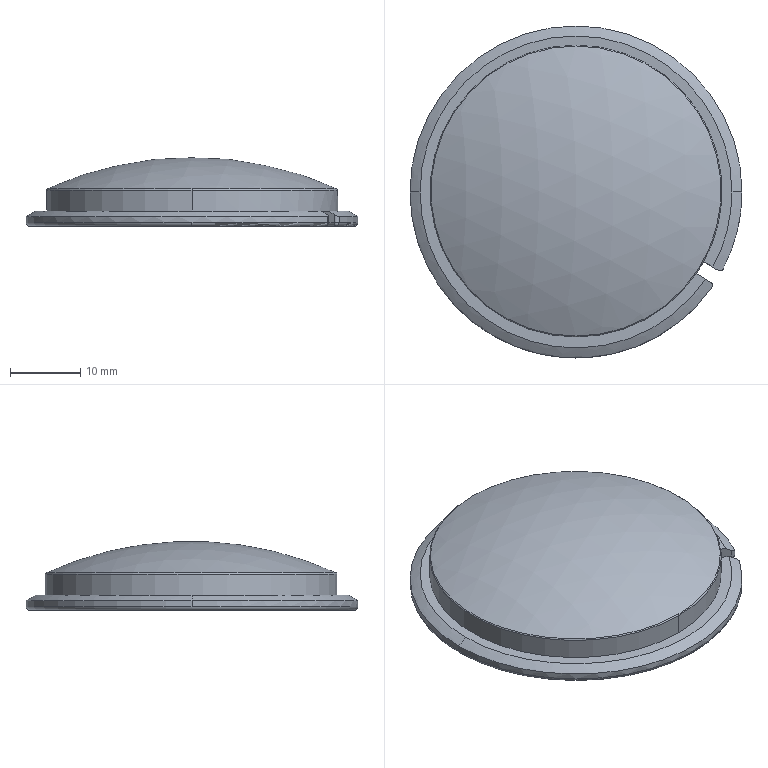Part | SolidWorks | features BaseBody 1 | 1 solid | 32 faces | box 47.34 x 47.34 x 9.8 mm | volume 4396 mm3 | torus 12 | cylinder 12 | plane 4 | sphere 4 | commonest cylinder face diameters 1 x5 47.34 x3 37.6 x2 41.6 x2
STEP:
#1=CARTESIAN_POINT('',(-125.381,-12.906,0.4856));
#2=VERTEX_POINT('',#1);
#3=CARTESIAN_POINT('',(-125.381,28.46,0.4856));
#4=VERTEX_POINT('',#3);
#5=CARTESIAN_POINT('',(-125.381,7.777,0.4856));
#6=DIRECTION('',(0.,0.,1.));
#7=DIRECTION('',(0.,1.,0.));
#8=AXIS2_PLACEMENT_3D('',#5,#6,#7);
#9=CIRCLE('',#8,20.683);
#10=EDGE_CURVE('',#2,#4,#9,.T.);
#11=ORIENTED_EDGE('',*,*,#10,.F.);
#12=CARTESIAN_POINT('',(-125.381,-13.023,0.3035));
#13=VERTEX_POINT('',#12);
#14=CARTESIAN_POINT('',(-125.381,-12.823,0.3035));
#15=DIRECTION('',(1.,0.,0.));
#16=DIRECTION('',(0.,1.,0.));
#17=AXIS2_PLACEMENT_3D('',#14,#15,#16);
#18=CIRCLE('',#17,0.2);
#19=EDGE_CURVE('',#2,#13,#18,.T.);
#20=ORIENTED_EDGE('',*,*,#19,.T.);
#21=CARTESIAN_POINT('',(-125.381,28.577,0.3035));
#22=VERTEX_POINT('',#21);
#23=CARTESIAN_POINT('',(-125.381,7.777,0.3035));
#24=DIRECTION('',(0.,0.,1.));
#25=DIRECTION('',(0.,-1.,0.));
#26=AXIS2_PLACEMENT_3D('',#23,#24,#25);
#27=CIRCLE('',#26,20.8);
#28=EDGE_CURVE('',#13,#22,#27,.T.);
#29=ORIENTED_EDGE('',*,*,#28,.T.);
#30=CARTESIAN_POINT('',(-125.381,28.377,0.3035));
#31=DIRECTION('',(-1.,0.,0.));
#32=DIRECTION('',(0.,0.,1.));
#33=AXIS2_PLACEMENT_3D('',#30,#31,#32);
#34=CIRCLE('',#33,0.2);
#35=EDGE_CURVE('',#4,#22,#34,.T.);
#36=ORIENTED_EDGE('',*,*,#35,.F.);
#37=EDGE_LOOP('',(#11,#20,#29,#36));
#38=FACE_OUTER_BOUND('',#37,.T.);
#39=CARTESIAN_POINT('',(-125.381,7.777,0.3035));
#40=DIRECTION('',(0.,0.,-1.));
#41=DIRECTION('',(0.,1.,0.));
#42=AXIS2_PLACEMENT_3D('',#39,#40,#41);
#43=TOROIDAL_SURFACE('',#42,20.6,0.2);
#44=ADVANCED_FACE('',(#38),#43,.T.);
#45=ORIENTED_EDGE('',*,*,#28,.F.);
#46=CARTESIAN_POINT('',(-125.381,-13.023,-2.679));
#47=VERTEX_POINT('',#46);
#48=CARTESIAN_POINT('',(-125.381,-13.023,4.965));
#49=DIRECTION('',(0.,0.,-1.));
#50=VECTOR('',#49,1000.);
#51=LINE('',#48,#50);
#52=EDGE_CURVE('',#13,#47,#51,.T.);
#53=ORIENTED_EDGE('',*,*,#52,.T.);
#54=CARTESIAN_POINT('',(-108.216,-3.971,-2.679));
#55=VERTEX_POINT('',#54);
#56=CARTESIAN_POINT('',(-125.381,7.777,-2.679));
#57=DIRECTION('',(0.,0.,1.));
#58=DIRECTION('',(0.,1.,0.));
#59=AXIS2_PLACEMENT_3D('',#56,#57,#58);
#60=CIRCLE('',#59,20.8);
#61=EDGE_CURVE('',#47,#55,#60,.T.);
#62=ORIENTED_EDGE('',*,*,#61,.T.);
#63=CARTESIAN_POINT('',(-108.216,-3.971,-4.336));
#64=VERTEX_POINT('',#63);
#65=CARTESIAN_POINT('',(-108.216,-3.971,-16.89));
#66=DIRECTION('',(0.,0.,-1.));
#67=VECTOR('',#66,1000.);
#68=LINE('',#65,#67);
#69=EDGE_CURVE('',#55,#64,#68,.T.);
#70=ORIENTED_EDGE('',*,*,#69,.T.);
#71=CARTESIAN_POINT('',(-108.504,-4.381,-4.836));
#72=VERTEX_POINT('',#71);
#73=CARTESIAN_POINT('',(-108.504,-4.381,-4.836));
#74=CARTESIAN_POINT('',(-108.427,-4.273,-4.836));
#75=CARTESIAN_POINT('',(-108.352,-4.168,-4.782));
#76=CARTESIAN_POINT('',(-108.247,-4.016,-4.598));
#77=CARTESIAN_POINT('',(-108.216,-3.971,-4.468));
#78=CARTESIAN_POINT('',(-108.216,-3.971,-4.336));
#79=B_SPLINE_CURVE_WITH_KNOTS('',3,(#73,#74,#75,#76,#77,#78),.UNSPECIFIED.,.F.,.F.,(4,2,4),(0.,0.0003909,0.0007818),.UNSPECIFIED.);
#80=EDGE_CURVE('',#72,#64,#79,.T.);
#81=ORIENTED_EDGE('',*,*,#80,.F.);
#82=CARTESIAN_POINT('',(-106.931,-1.826,-4.836));
#83=VERTEX_POINT('',#82);
#84=CARTESIAN_POINT('',(-125.381,7.777,-4.836));
#85=DIRECTION('',(0.,0.,1.));
#86=DIRECTION('',(0.,1.,0.));
#87=AXIS2_PLACEMENT_3D('',#84,#85,#86);
#88=CIRCLE('',#87,20.8);
#89=EDGE_CURVE('',#72,#83,#88,.T.);
#90=ORIENTED_EDGE('',*,*,#89,.T.);
#91=CARTESIAN_POINT('',(-107.167,-2.268,-4.336));
#92=VERTEX_POINT('',#91);
#93=CARTESIAN_POINT('',(-107.167,-2.268,-4.336));
#94=CARTESIAN_POINT('',(-107.167,-2.268,-4.468));
#95=CARTESIAN_POINT('',(-107.141,-2.22,-4.598));
#96=CARTESIAN_POINT('',(-107.053,-2.058,-4.782));
#97=CARTESIAN_POINT('',(-106.992,-1.944,-4.836));
#98=CARTESIAN_POINT('',(-106.931,-1.826,-4.836));
#99=B_SPLINE_CURVE_WITH_KNOTS('',3,(#93,#94,#95,#96,#97,#98),.UNSPECIFIED.,.F.,.F.,(4,2,4),(0.,0.0003909,0.0007818),.UNSPECIFIED.);
#100=EDGE_CURVE('',#92,#83,#99,.T.);
#101=ORIENTED_EDGE('',*,*,#100,.F.);
#102=CARTESIAN_POINT('',(-107.167,-2.268,-2.679));
#103=VERTEX_POINT('',#102);
#104=CARTESIAN_POINT('',(-107.167,-2.268,-16.89));
#105=DIRECTION('',(0.,0.,1.));
#106=VECTOR('',#105,1000.);
#107=LINE('',#104,#106);
#108=EDGE_CURVE('',#92,#103,#107,.T.);
#109=ORIENTED_EDGE('',*,*,#108,.T.);
#110=CARTESIAN_POINT('',(-125.381,28.577,-2.679));
#111=VERTEX_POINT('',#110);
#112=CARTESIAN_POINT('',(-125.381,7.777,-2.679));
#113=DIRECTION('',(0.,0.,1.));
#114=DIRECTION('',(0.,1.,0.));
#115=AXIS2_PLACEMENT_3D('',#112,#113,#114);
#116=CIRCLE('',#115,20.8);
#117=EDGE_CURVE('',#103,#111,#116,.T.);
#118=ORIENTED_EDGE('',*,*,#117,.T.);
#119=CARTESIAN_POINT('',(-125.381,28.577,4.965));
#120=DIRECTION('',(0.,0.,-1.));
#121=VECTOR('',#120,1000.);
#122=LINE('',#119,#121);
#123=EDGE_CURVE('',#22,#111,#122,.T.);
#124=ORIENTED_EDGE('',*,*,#123,.F.);
#125=EDGE_LOOP('',(#45,#53,#62,#70,#81,#90,#101,#109,#118,#124));
#126=FACE_OUTER_BOUND('',#125,.T.);
#127=CARTESIAN_POINT('',(-125.381,7.777,4.965));
#128=DIRECTION('',(0.,0.,-1.));
#129=DIRECTION('',(0.,1.,0.));
#130=AXIS2_PLACEMENT_3D('',#127,#128,#129);
#131=CYLINDRICAL_SURFACE('',#130,20.8);
#132=ADVANCED_FACE('',(#126),#131,.T.);
#133=CARTESIAN_POINT('',(-125.381,-11.023,-2.836));
#134=VERTEX_POINT('',#133);
#135=CARTESIAN_POINT('',(-125.381,26.577,-2.836));
#136=VERTEX_POINT('',#135);
#137=CARTESIAN_POINT('',(-125.381,7.777,-2.836));
#138=DIRECTION('',(0.,0.,1.));
#139=DIRECTION('',(0.,-1.,0.));
#140=AXIS2_PLACEMENT_3D('',#137,#138,#139);
#141=CIRCLE('',#140,18.8);
#142=EDGE_CURVE('',#134,#136,#141,.T.);
#143=ORIENTED_EDGE('',*,*,#142,.T.);
#144=CARTESIAN_POINT('',(-125.381,28.577,-4.836));
#145=VERTEX_POINT('',#144);
#146=CARTESIAN_POINT('',(-125.381,28.577,-2.836));
#147=DIRECTION('',(1.,0.,0.));
#148=DIRECTION('',(0.,1.,0.));
#149=AXIS2_PLACEMENT_3D('',#146,#147,#148);
#150=CIRCLE('',#149,2.);
#151=EDGE_CURVE('',#136,#145,#150,.T.);
#152=ORIENTED_EDGE('',*,*,#151,.T.);
#153=CARTESIAN_POINT('',(-125.381,7.777,-4.836));
#154=DIRECTION('',(0.,0.,-1.));
#155=DIRECTION('',(0.,-1.,0.));
#156=AXIS2_PLACEMENT_3D('',#153,#154,#155);
#157=CIRCLE('',#156,20.8);
#158=EDGE_CURVE('',#145,#83,#157,.T.);
#159=ORIENTED_EDGE('',*,*,#158,.T.);
#160=ORIENTED_EDGE('',*,*,#89,.F.);
#161=CARTESIAN_POINT('',(-125.381,-13.023,-4.836));
#162=VERTEX_POINT('',#161);
#163=CARTESIAN_POINT('',(-125.381,7.777,-4.836));
#164=DIRECTION('',(0.,0.,-1.));
#165=DIRECTION('',(0.,-1.,0.));
#166=AXIS2_PLACEMENT_3D('',#163,#164,#165);
#167=CIRCLE('',#166,20.8);
#168=EDGE_CURVE('',#72,#162,#167,.T.);
#169=ORIENTED_EDGE('',*,*,#168,.T.);
#170=CARTESIAN_POINT('',(-125.381,-13.023,-2.836));
#171=DIRECTION('',(-1.,0.,0.));
#172=DIRECTION('',(0.,0.,1.));
#173=AXIS2_PLACEMENT_3D('',#170,#171,#172);
#174=CIRCLE('',#173,2.);
#175=EDGE_CURVE('',#134,#162,#174,.T.);
#176=ORIENTED_EDGE('',*,*,#175,.F.);
#177=EDGE_LOOP('',(#143,#152,#159,#160,#169,#176));
#178=FACE_OUTER_BOUND('',#177,.T.);
#179=CARTESIAN_POINT('',(-125.381,7.777,-2.836));
#180=DIRECTION('',(0.,0.,1.));
#181=DIRECTION('',(0.,-1.,0.));
#182=AXIS2_PLACEMENT_3D('',#179,#180,#181);
#183=TOROIDAL_SURFACE('',#182,20.8,2.);
#184=ADVANCED_FACE('',(#178),#183,.T.);
#185=CARTESIAN_POINT('',(-101.711,7.647,-3.467));
#186=VERTEX_POINT('',#185);
#187=CARTESIAN_POINT('',(-149.051,7.647,-3.467));
#188=VERTEX_POINT('',#187);
#189=CARTESIAN_POINT('',(-125.381,7.647,-3.467));
#190=DIRECTION('',(0.,0.,1.));
#191=DIRECTION('',(0.,-1.,0.));
#192=AXIS2_PLACEMENT_3D('',#189,#190,#191);
#193=CIRCLE('',#192,23.67);
#194=EDGE_CURVE('',#186,#188,#193,.T.);
#195=ORIENTED_EDGE('',*,*,#194,.T.);
#196=CARTESIAN_POINT('',(-147.618,7.647,-2.679));
#197=VERTEX_POINT('',#196);
#198=CARTESIAN_POINT('',(-125.251,7.647,-45.036));
#199=DIRECTION('',(0.,1.,0.));
#200=DIRECTION('',(-1.,0.,0.));
#201=AXIS2_PLACEMENT_3D('',#198,#199,#200);
#202=CIRCLE('',#201,47.9);
#203=EDGE_CURVE('',#188,#197,#202,.T.);
#204=ORIENTED_EDGE('',*,*,#203,.T.);
#205=CARTESIAN_POINT('',(-103.144,7.647,-2.679));
#206=VERTEX_POINT('',#205);
#207=CARTESIAN_POINT('',(-125.381,7.647,-2.679));
#208=DIRECTION('',(0.,0.,1.));
#209=DIRECTION('',(1.,0.,0.));
#210=AXIS2_PLACEMENT_3D('',#207,#208,#209);
#211=CIRCLE('',#210,22.237);
#212=EDGE_CURVE('',#206,#197,#211,.T.);
#213=ORIENTED_EDGE('',*,*,#212,.F.);
#214=CARTESIAN_POINT('',(-125.511,7.647,-45.036));
#215=DIRECTION('',(0.,-1.,0.));
#216=DIRECTION('',(0.,0.,-1.));
#217=AXIS2_PLACEMENT_3D('',#214,#215,#216);
#218=CIRCLE('',#217,47.9);
#219=EDGE_CURVE('',#186,#206,#218,.T.);
#220=ORIENTED_EDGE('',*,*,#219,.F.);
#221=EDGE_LOOP('',(#195,#204,#213,#220));
#222=FACE_OUTER_BOUND('',#221,.T.);
#223=CARTESIAN_POINT('',(-125.381,7.647,-45.036));
#224=DIRECTION('',(0.,0.,1.));
#225=DIRECTION('',(1.,0.,0.));
#226=AXIS2_PLACEMENT_3D('',#223,#224,#225);
#227=TOROIDAL_SURFACE('',#226,-0.1299,47.9);
#228=ADVANCED_FACE('',(#222),#227,.T.);
#229=CARTESIAN_POINT('',(-104.413,-3.336,-3.467));
#230=VERTEX_POINT('',#229);
#231=CARTESIAN_POINT('',(-125.381,7.647,-3.467));
#232=DIRECTION('',(0.,0.,1.));
#233=DIRECTION('',(0.,-1.,0.));
#234=AXIS2_PLACEMENT_3D('',#231,#232,#233);
#235=CIRCLE('',#234,23.67);
#236=EDGE_CURVE('',#230,#186,#235,.T.);
#237=ORIENTED_EDGE('',*,*,#236,.T.);
#238=ORIENTED_EDGE('',*,*,#219,.T.);
#239=CARTESIAN_POINT('',(-105.889,-3.055,-2.679));
#240=VERTEX_POINT('',#239);
#241=CARTESIAN_POINT('',(-125.381,7.647,-2.679));
#242=DIRECTION('',(0.,0.,1.));
#243=DIRECTION('',(1.,0.,0.));
#244=AXIS2_PLACEMENT_3D('',#241,#242,#243);
#245=CIRCLE('',#244,22.237);
#246=EDGE_CURVE('',#240,#206,#245,.T.);
#247=ORIENTED_EDGE('',*,*,#246,.F.);
#248=CARTESIAN_POINT('',(-105.119,-3.53,-3.169));
#249=VERTEX_POINT('',#248);
#250=CARTESIAN_POINT('',(-105.889,-3.055,-2.679));
#251=CARTESIAN_POINT('',(-105.636,-3.211,-2.836));
#252=CARTESIAN_POINT('',(-105.379,-3.369,-2.999));
#253=CARTESIAN_POINT('',(-105.119,-3.53,-3.169));
#254=B_SPLINE_CURVE_WITH_KNOTS('',3,(#250,#251,#252,#253),.UNSPECIFIED.,.F.,.F.,(4,4),(0.,1.),.UNSPECIFIED.);
#255=EDGE_CURVE('',#240,#249,#254,.T.);
#256=ORIENTED_EDGE('',*,*,#255,.T.);
#257=CARTESIAN_POINT('',(-105.119,-3.53,-3.169));
#258=CARTESIAN_POINT('',(-105.063,-3.564,-3.205));
#259=CARTESIAN_POINT('',(-105.004,-3.586,-3.24));
#260=CARTESIAN_POINT('',(-104.875,-3.608,-3.309));
#261=CARTESIAN_POINT('',(-104.808,-3.606,-3.342));
#262=CARTESIAN_POINT('',(-104.676,-3.575,-3.399));
#263=CARTESIAN_POINT('',(-104.612,-3.546,-3.423));
#264=CARTESIAN_POINT('',(-104.497,-3.459,-3.458));
#265=CARTESIAN_POINT('',(-104.448,-3.402,-3.467));
#266=CARTESIAN_POINT('',(-104.413,-3.336,-3.467));
#267=B_SPLINE_CURVE_WITH_KNOTS('',3,(#257,#258,#259,#260,#261,#262,#263,#264,#265,#266),.UNSPECIFIED.,.F.,.F.,(4,2,2,2,4),(0.,0.0002187,0.0004373,0.000656,0.0008747),.UNSPECIFIED.);
#268=EDGE_CURVE('',#249,#230,#267,.T.);
#269=ORIENTED_EDGE('',*,*,#268,.T.);
#270=EDGE_LOOP('',(#237,#238,#247,#256,#269));
#271=FACE_OUTER_BOUND('',#270,.T.);
#272=CARTESIAN_POINT('',(-125.381,7.647,-45.036));
#273=DIRECTION('',(0.,0.,1.));
#274=DIRECTION('',(1.,0.,0.));
#275=AXIS2_PLACEMENT_3D('',#272,#273,#274);
#276=TOROIDAL_SURFACE('',#275,-0.1299,47.9);
#277=ADVANCED_FACE('',(#271),#276,.T.);
#278=CARTESIAN_POINT('',(-125.381,-11.023,-1.537));
#279=VERTEX_POINT('',#278);
#280=CARTESIAN_POINT('',(-125.381,26.577,-1.537));
#281=VERTEX_POINT('',#280);
#282=CARTESIAN_POINT('',(-125.381,7.777,-1.537));
#283=DIRECTION('',(0.,0.,-1.));
#284=DIRECTION('',(0.,1.,0.));
#285=AXIS2_PLACEMENT_3D('',#282,#283,#284);
#286=CIRCLE('',#285,18.8);
#287=EDGE_CURVE('',#279,#281,#286,.T.);
#288=ORIENTED_EDGE('',*,*,#287,.F.);
#289=CARTESIAN_POINT('',(-125.381,-11.023,4.965));
#290=DIRECTION('',(0.,0.,-1.));
#291=VECTOR('',#290,1000.);
#292=LINE('',#289,#291);
#293=EDGE_CURVE('',#279,#134,#292,.T.);
#294=ORIENTED_EDGE('',*,*,#293,.T.);
#295=CARTESIAN_POINT('',(-125.381,7.777,-2.836));
#296=DIRECTION('',(0.,0.,1.));
#297=DIRECTION('',(0.,-1.,0.));
#298=AXIS2_PLACEMENT_3D('',#295,#296,#297);
#299=CIRCLE('',#298,18.8);
#300=EDGE_CURVE('',#136,#134,#299,.T.);
#301=ORIENTED_EDGE('',*,*,#300,.F.);
#302=CARTESIAN_POINT('',(-125.381,26.577,4.965));
#303=DIRECTION('',(0.,0.,-1.));
#304=VECTOR('',#303,1000.);
#305=LINE('',#302,#304);
#306=EDGE_CURVE('',#281,#136,#305,.T.);
#307=ORIENTED_EDGE('',*,*,#306,.F.);
#308=EDGE_LOOP('',(#288,#294,#301,#307));
#309=FACE_OUTER_BOUND('',#308,.T.);
#310=CARTESIAN_POINT('',(-125.381,7.777,4.965));
#311=DIRECTION('',(0.,0.,-1.));
#312=DIRECTION('',(0.,1.,0.));
#313=AXIS2_PLACEMENT_3D('',#310,#311,#312);
#314=CYLINDRICAL_SURFACE('',#313,18.8);
#315=ADVANCED_FACE('',(#309),#314,.F.);
#316=CARTESIAN_POINT('',(-106.008,-5.953,-4.336));
#317=VERTEX_POINT('',#316);
#318=CARTESIAN_POINT('',(-105.918,-5.666,-4.336));
#319=VERTEX_POINT('',#318);
#320=CARTESIAN_POINT('',(-106.418,-5.666,-4.336));
#321=DIRECTION('',(0.,0.,1.));
#322=DIRECTION('',(1.,0.,0.));
#323=AXIS2_PLACEMENT_3D('',#320,#321,#322);
#324=CIRCLE('',#323,0.5);
#325=EDGE_CURVE('',#317,#319,#324,.T.);
#326=ORIENTED_EDGE('',*,*,#325,.T.);
#327=CARTESIAN_POINT('',(-105.918,-5.666,-3.416));
#328=VERTEX_POINT('',#327);
#329=CARTESIAN_POINT('',(-105.918,-5.666,4.5));
#330=DIRECTION('',(0.,0.,1.));
#331=VECTOR('',#330,1000.);
#332=LINE('',#329,#331);
#333=EDGE_CURVE('',#319,#328,#332,.T.);
#334=ORIENTED_EDGE('',*,*,#333,.T.);
#335=CARTESIAN_POINT('',(-106.008,-5.953,-3.467));
#336=VERTEX_POINT('',#335);
#337=CARTESIAN_POINT('',(-106.008,-5.953,-3.467));
#338=CARTESIAN_POINT('',(-105.948,-5.867,-3.467));
#339=CARTESIAN_POINT('',(-105.918,-5.766,-3.448));
#340=CARTESIAN_POINT('',(-105.918,-5.666,-3.416));
#341=B_SPLINE_CURVE_WITH_KNOTS('',3,(#337,#338,#339,#340),.UNSPECIFIED.,.F.,.F.,(4,4),(-0.0003094,0.),.UNSPECIFIED.);
#342=EDGE_CURVE('',#336,#328,#341,.T.);
#343=ORIENTED_EDGE('',*,*,#342,.F.);
#344=CARTESIAN_POINT('',(-106.008,-5.953,4.5));
#345=DIRECTION('',(0.,0.,-1.));
#346=VECTOR('',#345,1000.);
#347=LINE('',#344,#346);
#348=EDGE_CURVE('',#336,#317,#347,.T.);
#349=ORIENTED_EDGE('',*,*,#348,.T.);
#350=EDGE_LOOP('',(#326,#334,#343,#349));
#351=FACE_OUTER_BOUND('',#350,.T.);
#352=CARTESIAN_POINT('',(-106.418,-5.666,4.5));
#353=DIRECTION('',(0.,0.,1.));
#354=DIRECTION('',(1.,0.,0.));
#355=AXIS2_PLACEMENT_3D('',#352,#353,#354);
#356=CYLINDRICAL_SURFACE('',#355,0.5);
#357=ADVANCED_FACE('',(#351),#356,.T.);
#358=CARTESIAN_POINT('',(-125.381,31.317,-4.336));
#359=VERTEX_POINT('',#358);
#360=CARTESIAN_POINT('',(-149.051,7.647,-4.336));
#361=VERTEX_POINT('',#360);
#362=CARTESIAN_POINT('',(-125.381,7.647,-4.336));
#363=DIRECTION('',(0.,0.,1.));
#364=DIRECTION('',(1.,0.,0.));
#365=AXIS2_PLACEMENT_3D('',#362,#363,#364);
#366=CIRCLE('',#365,23.67);
#367=EDGE_CURVE('',#359,#361,#366,.T.);
#368=ORIENTED_EDGE('',*,*,#367,.T.);
#369=CARTESIAN_POINT('',(-149.051,7.647,4.5));
#370=DIRECTION('',(0.,0.,1.));
#371=VECTOR('',#370,1000.);
#372=LINE('',#369,#371);
#373=EDGE_CURVE('',#361,#188,#372,.T.);
#374=ORIENTED_EDGE('',*,*,#373,.T.);
#375=ORIENTED_EDGE('',*,*,#194,.F.);
#376=CARTESIAN_POINT('',(-101.711,7.647,-4.336));
#377=VERTEX_POINT('',#376);
#378=CARTESIAN_POINT('',(-101.711,7.647,4.5));
#379=DIRECTION('',(0.,0.,1.));
#380=VECTOR('',#379,1000.);
#381=LINE('',#378,#380);
#382=EDGE_CURVE('',#377,#186,#381,.T.);
#383=ORIENTED_EDGE('',*,*,#382,.F.);
#384=CARTESIAN_POINT('',(-125.381,7.647,-4.336));
#385=DIRECTION('',(0.,0.,1.));
#386=DIRECTION('',(1.,0.,0.));
#387=AXIS2_PLACEMENT_3D('',#384,#385,#386);
#388=CIRCLE('',#387,23.67);
#389=EDGE_CURVE('',#377,#359,#388,.T.);
#390=ORIENTED_EDGE('',*,*,#389,.T.);
#391=EDGE_LOOP('',(#368,#374,#375,#383,#390));
#392=FACE_OUTER_BOUND('',#391,.T.);
#393=CARTESIAN_POINT('',(-125.381,7.647,4.5));
#394=DIRECTION('',(0.,0.,1.));
#395=DIRECTION('',(1.,0.,0.));
#396=AXIS2_PLACEMENT_3D('',#393,#394,#395);
#397=CYLINDRICAL_SURFACE('',#396,23.67);
#398=ADVANCED_FACE('',(#392),#397,.T.);
#399=CARTESIAN_POINT('',(-104.413,-3.336,-4.336));
#400=VERTEX_POINT('',#399);
#401=CARTESIAN_POINT('',(-125.381,7.647,-4.336));
#402=DIRECTION('',(0.,0.,1.));
#403=DIRECTION('',(1.,0.,0.));
#404=AXIS2_PLACEMENT_3D('',#401,#402,#403);
#405=CIRCLE('',#404,23.67);
#406=EDGE_CURVE('',#400,#377,#405,.T.);
#407=ORIENTED_EDGE('',*,*,#406,.T.);
#408=ORIENTED_EDGE('',*,*,#382,.T.);
#409=ORIENTED_EDGE('',*,*,#236,.F.);
#410=CARTESIAN_POINT('',(-104.413,-3.336,4.5));
#411=DIRECTION('',(0.,0.,-1.));
#412=VECTOR('',#411,1000.);
#413=LINE('',#410,#412);
#414=EDGE_CURVE('',#230,#400,#413,.T.);
#415=ORIENTED_EDGE('',*,*,#414,.T.);
#416=EDGE_LOOP('',(#407,#408,#409,#415));
#417=FACE_OUTER_BOUND('',#416,.T.);
#418=CARTESIAN_POINT('',(-125.381,7.647,4.5));
#419=DIRECTION('',(0.,0.,1.));
#420=DIRECTION('',(1.,0.,0.));
#421=AXIS2_PLACEMENT_3D('',#418,#419,#420);
#422=CYLINDRICAL_SURFACE('',#421,23.67);
#423=ADVANCED_FACE('',(#417),#422,.T.);
#424=CARTESIAN_POINT('',(-104.856,-3.104,-4.836));
#425=VERTEX_POINT('',#424);
#426=CARTESIAN_POINT('',(-125.381,30.817,-4.836));
#427=VERTEX_POINT('',#426);
#428=CARTESIAN_POINT('',(-125.381,7.647,-4.836));
#429=DIRECTION('',(0.,0.,1.));
#430=DIRECTION('',(0.,-1.,0.));
#431=AXIS2_PLACEMENT_3D('',#428,#429,#430);
#432=CIRCLE('',#431,23.17);
#433=EDGE_CURVE('',#425,#427,#432,.T.);
#434=ORIENTED_EDGE('',*,*,#433,.T.);
#435=CARTESIAN_POINT('',(-125.381,30.817,-4.336));
#436=DIRECTION('',(1.,0.,0.));
#437=DIRECTION('',(0.,1.,0.));
#438=AXIS2_PLACEMENT_3D('',#435,#436,#437);
#439=CIRCLE('',#438,0.5);
#440=EDGE_CURVE('',#427,#359,#439,.T.);
#441=ORIENTED_EDGE('',*,*,#440,.T.);
#442=ORIENTED_EDGE('',*,*,#389,.F.);
#443=ORIENTED_EDGE('',*,*,#406,.F.);
#444=CARTESIAN_POINT('',(-104.856,-3.104,-4.336));
#445=DIRECTION('',(0.464,0.8858,0.));
#446=DIRECTION('',(-0.8858,0.464,0.));
#447=AXIS2_PLACEMENT_3D('',#444,#445,#446);
#448=CIRCLE('',#447,0.5);
#449=EDGE_CURVE('',#400,#425,#448,.T.);
#450=ORIENTED_EDGE('',*,*,#449,.T.);
#451=EDGE_LOOP('',(#434,#441,#442,#443,#450));
#452=FACE_OUTER_BOUND('',#451,.T.);
#453=CARTESIAN_POINT('',(-125.381,7.647,-4.336));
#454=DIRECTION('',(0.,0.,1.));
#455=DIRECTION('',(0.,-1.,0.));
#456=AXIS2_PLACEMENT_3D('',#453,#454,#455);
#457=TOROIDAL_SURFACE('',#456,23.17,0.5);
#458=ADVANCED_FACE('',(#452),#457,.T.);
#459=ORIENTED_EDGE('',*,*,#440,.F.);
#460=CARTESIAN_POINT('',(-125.381,-15.523,-4.836));
#461=VERTEX_POINT('',#460);
#462=CARTESIAN_POINT('',(-125.381,7.647,-4.836));
#463=DIRECTION('',(0.,0.,1.));
#464=DIRECTION('',(0.,-1.,0.));
#465=AXIS2_PLACEMENT_3D('',#462,#463,#464);
#466=CIRCLE('',#465,23.17);
#467=EDGE_CURVE('',#427,#461,#466,.T.);
#468=ORIENTED_EDGE('',*,*,#467,.T.);
#469=CARTESIAN_POINT('',(-125.381,-16.023,-4.336));
#470=VERTEX_POINT('',#469);
#471=CARTESIAN_POINT('',(-125.381,-15.523,-4.336));
#472=DIRECTION('',(-1.,0.,0.));
#473=DIRECTION('',(0.,0.,1.));
#474=AXIS2_PLACEMENT_3D('',#471,#472,#473);
#475=CIRCLE('',#474,0.5);
#476=EDGE_CURVE('',#461,#470,#475,.T.);
#477=ORIENTED_EDGE('',*,*,#476,.T.);
#478=CARTESIAN_POINT('',(-125.381,7.647,-4.336));
#479=DIRECTION('',(0.,0.,1.));
#480=DIRECTION('',(1.,0.,0.));
#481=AXIS2_PLACEMENT_3D('',#478,#479,#480);
#482=CIRCLE('',#481,23.67);
#483=EDGE_CURVE('',#361,#470,#482,.T.);
#484=ORIENTED_EDGE('',*,*,#483,.F.);
#485=ORIENTED_EDGE('',*,*,#367,.F.);
#486=EDGE_LOOP('',(#459,#468,#477,#484,#485));
#487=FACE_OUTER_BOUND('',#486,.T.);
#488=CARTESIAN_POINT('',(-125.381,7.647,-4.336));
#489=DIRECTION('',(0.,0.,1.));
#490=DIRECTION('',(0.,-1.,0.));
#491=AXIS2_PLACEMENT_3D('',#488,#489,#490);
#492=TOROIDAL_SURFACE('',#491,23.17,0.5);
#493=ADVANCED_FACE('',(#487),#492,.T.);
#494=CARTESIAN_POINT('',(-125.381,-10.402,-0.6116));
#495=VERTEX_POINT('',#494);
#496=CARTESIAN_POINT('',(-125.381,25.956,-0.6116));
#497=VERTEX_POINT('',#496);
#498=CARTESIAN_POINT('',(-125.381,7.777,-0.6116));
#499=DIRECTION('',(0.,0.,-1.));
#500=DIRECTION('',(0.,1.,0.));
#501=AXIS2_PLACEMENT_3D('',#498,#499,#500);
#502=CIRCLE('',#501,18.179);
#503=EDGE_CURVE('',#495,#497,#502,.T.);
#504=ORIENTED_EDGE('',*,*,#503,.F.);
#505=CARTESIAN_POINT('',(-125.381,-10.023,-1.537));
#506=DIRECTION('',(1.,0.,0.));
#507=DIRECTION('',(0.,1.,0.));
#508=AXIS2_PLACEMENT_3D('',#505,#506,#507);
#509=CIRCLE('',#508,1.);
#510=EDGE_CURVE('',#495,#279,#509,.T.);
#511=ORIENTED_EDGE('',*,*,#510,.T.);
#512=ORIENTED_EDGE('',*,*,#287,.T.);
#513=CARTESIAN_POINT('',(-125.381,25.577,-1.537));
#514=DIRECTION('',(-1.,0.,0.));
#515=DIRECTION('',(0.,0.,1.));
#516=AXIS2_PLACEMENT_3D('',#513,#514,#515);
#517=CIRCLE('',#516,1.);
#518=EDGE_CURVE('',#497,#281,#517,.T.);
#519=ORIENTED_EDGE('',*,*,#518,.F.);
#520=EDGE_LOOP('',(#504,#511,#512,#519));
#521=FACE_OUTER_BOUND('',#520,.T.);
#522=CARTESIAN_POINT('',(-125.381,7.777,-1.537));
#523=DIRECTION('',(0.,0.,-1.));
#524=DIRECTION('',(0.,1.,0.));
#525=AXIS2_PLACEMENT_3D('',#522,#523,#524);
#526=TOROIDAL_SURFACE('',#525,17.8,1.);
#527=ADVANCED_FACE('',(#521),#526,.F.);
#528=CARTESIAN_POINT('',(-125.381,7.777,0.4856));
#529=DIRECTION('',(0.,0.,1.));
#530=DIRECTION('',(0.,1.,0.));
#531=AXIS2_PLACEMENT_3D('',#528,#529,#530);
#532=CIRCLE('',#531,20.683);
#533=EDGE_CURVE('',#4,#2,#532,.T.);
#534=ORIENTED_EDGE('',*,*,#533,.T.);
#535=ORIENTED_EDGE('',*,*,#10,.T.);
#536=EDGE_LOOP('',(#534,#535));
#537=FACE_OUTER_BOUND('',#536,.T.);
#538=CARTESIAN_POINT('',(-125.381,7.777,-45.036));
#539=DIRECTION('',(-0.9094,0.,0.416));
#540=DIRECTION('',(0.416,0.,0.9094));
#541=AXIS2_PLACEMENT_3D('',#538,#539,#540);
#542=SPHERICAL_SURFACE('',#541,50.);
#543=ADVANCED_FACE('',(#537),#542,.T.);
#544=ORIENTED_EDGE('',*,*,#19,.F.);
#545=ORIENTED_EDGE('',*,*,#533,.F.);
#546=ORIENTED_EDGE('',*,*,#35,.T.);
#547=CARTESIAN_POINT('',(-125.381,7.777,0.3035));
#548=DIRECTION('',(0.,0.,1.));
#549=DIRECTION('',(0.,-1.,0.));
#550=AXIS2_PLACEMENT_3D('',#547,#548,#549);
#551=CIRCLE('',#550,20.8);
#552=EDGE_CURVE('',#22,#13,#551,.T.);
#553=ORIENTED_EDGE('',*,*,#552,.T.);
#554=EDGE_LOOP('',(#544,#545,#546,#553));
#555=FACE_OUTER_BOUND('',#554,.T.);
#556=CARTESIAN_POINT('',(-125.381,7.777,0.3035));
#557=DIRECTION('',(0.,0.,-1.));
#558=DIRECTION('',(0.,1.,0.));
#559=AXIS2_PLACEMENT_3D('',#556,#557,#558);
#560=TOROIDAL_SURFACE('',#559,20.6,0.2);
#561=ADVANCED_FACE('',(#555),#560,.T.);
#562=ORIENTED_EDGE('',*,*,#52,.F.);
#563=ORIENTED_EDGE('',*,*,#552,.F.);
#564=ORIENTED_EDGE('',*,*,#123,.T.);
#565=CARTESIAN_POINT('',(-125.381,7.777,-2.679));
#566=DIRECTION('',(0.,0.,1.));
#567=DIRECTION('',(0.,1.,0.));
#568=AXIS2_PLACEMENT_3D('',#565,#566,#567);
#569=CIRCLE('',#568,20.8);
#570=EDGE_CURVE('',#111,#47,#569,.T.);
#571=ORIENTED_EDGE('',*,*,#570,.T.);
#572=EDGE_LOOP('',(#562,#563,#564,#571));
#573=FACE_OUTER_BOUND('',#572,.T.);
#574=CARTESIAN_POINT('',(-125.381,7.777,4.965));
#575=DIRECTION('',(0.,0.,-1.));
#576=DIRECTION('',(0.,1.,0.));
#577=AXIS2_PLACEMENT_3D('',#574,#575,#576);
#578=CYLINDRICAL_SURFACE('',#577,20.8);
#579=ADVANCED_FACE('',(#573),#578,.T.);
#580=CARTESIAN_POINT('',(-106.929,-4.764,-2.679));
#581=VERTEX_POINT('',#580);
#582=CARTESIAN_POINT('',(-108.216,-3.971,-2.679));
#583=DIRECTION('',(-0.8514,0.5245,0.));
#584=VECTOR('',#583,1000.);
#585=LINE('',#582,#584);
#586=EDGE_CURVE('',#581,#55,#585,.T.);
#587=ORIENTED_EDGE('',*,*,#586,.T.);
#588=ORIENTED_EDGE('',*,*,#61,.F.);
#589=ORIENTED_EDGE('',*,*,#570,.F.);
#590=ORIENTED_EDGE('',*,*,#117,.F.);
#591=CARTESIAN_POINT('',(-107.167,-2.268,-2.679));
#592=DIRECTION('',(0.8514,-0.5245,0.));
#593=VECTOR('',#592,1000.);
#594=LINE('',#591,#593);
#595=EDGE_CURVE('',#103,#240,#594,.T.);
#596=ORIENTED_EDGE('',*,*,#595,.T.);
#597=ORIENTED_EDGE('',*,*,#246,.T.);
#598=ORIENTED_EDGE('',*,*,#212,.T.);
#599=CARTESIAN_POINT('',(-125.381,7.647,-2.679));
#600=DIRECTION('',(0.,0.,1.));
#601=DIRECTION('',(1.,0.,0.));
#602=AXIS2_PLACEMENT_3D('',#599,#600,#601);
#603=CIRCLE('',#602,22.237);
#604=EDGE_CURVE('',#197,#581,#603,.T.);
#605=ORIENTED_EDGE('',*,*,#604,.T.);
#606=EDGE_LOOP('',(#587,#588,#589,#590,#596,#597,#598,#605));
#607=FACE_OUTER_BOUND('',#606,.T.);
#608=CARTESIAN_POINT('',(-125.381,-14.59,-2.679));
#609=DIRECTION('',(0.,0.,1.));
#610=DIRECTION('',(1.,0.,0.));
#611=AXIS2_PLACEMENT_3D('',#608,#609,#610);
#612=PLANE('',#611);
#613=ADVANCED_FACE('',(#607),#612,.T.);
#614=ORIENTED_EDGE('',*,*,#151,.F.);
#615=ORIENTED_EDGE('',*,*,#300,.T.);
#616=ORIENTED_EDGE('',*,*,#175,.T.);
#617=CARTESIAN_POINT('',(-125.381,-13.023,-4.836));
#618=CARTESIAN_POINT('',(-126.484,-13.023,-4.836));
#619=CARTESIAN_POINT('',(-127.54,-12.935,-4.836));
#620=CARTESIAN_POINT('',(-129.535,-12.629,-4.836));
#621=CARTESIAN_POINT('',(-130.475,-12.41,-4.836));
#622=CARTESIAN_POINT('',(-132.229,-11.885,-4.836));
#623=CARTESIAN_POINT('',(-133.044,-11.577,-4.836));
#624=CARTESIAN_POINT('',(-134.548,-10.912,-4.836));
#625=CARTESIAN_POINT('',(-135.237,-10.554,-4.836));
#626=CARTESIAN_POINT('',(-137.125,-9.452,-4.836));
#627=CARTESIAN_POINT('',(-138.144,-8.683,-4.836));
#628=CARTESIAN_POINT('',(-139.785,-7.268,-4.836));
#629=CARTESIAN_POINT('',(-140.408,-6.622,-4.836));
#630=CARTESIAN_POINT('',(-141.354,-5.565,-4.836));
#631=CARTESIAN_POINT('',(-141.677,-5.154,-4.836));
#632=CARTESIAN_POINT('',(-141.931,-4.823,-4.836));
#633=CARTESIAN_POINT('',(-141.975,-4.765,-4.836));
#634=CARTESIAN_POINT('',(-142.02,-4.705,-4.836));
#635=CARTESIAN_POINT('',(-142.031,-4.691,-4.836));
#636=CARTESIAN_POINT('',(-142.041,-4.676,-4.836));
#637=CARTESIAN_POINT('',(-142.044,-4.673,-4.836));
#638=CARTESIAN_POINT('',(-142.045,-4.672,-4.836));
#639=CARTESIAN_POINT('',(-142.045,-4.672,-4.836));
#640=CARTESIAN_POINT('',(-142.049,-4.667,-4.836));
#641=CARTESIAN_POINT('',(-142.058,-4.655,-4.836));
#642=CARTESIAN_POINT('',(-142.096,-4.603,-4.836));
#643=CARTESIAN_POINT('',(-142.25,-4.394,-4.836));
#644=CARTESIAN_POINT('',(-142.621,-3.872,-4.836));
#645=CARTESIAN_POINT('',(-142.943,-3.376,-4.836));
#646=CARTESIAN_POINT('',(-143.251,-2.87,-4.836));
#647=CARTESIAN_POINT('',(-143.401,-2.616,-4.836));
#648=CARTESIAN_POINT('',(-143.57,-2.315,-4.836));
#649=CARTESIAN_POINT('',(-143.652,-2.163,-4.836));
#650=CARTESIAN_POINT('',(-143.687,-2.098,-4.836));
#651=CARTESIAN_POINT('',(-143.711,-2.055,-4.836));
#652=CARTESIAN_POINT('',(-143.722,-2.034,-4.836));
#653=CARTESIAN_POINT('',(-143.931,-1.642,-4.836));
#654=CARTESIAN_POINT('',(-144.117,-1.267,-4.836));
#655=CARTESIAN_POINT('',(-144.335,-0.7911,-4.836));
#656=CARTESIAN_POINT('',(-144.389,-0.6718,-4.836));
#657=CARTESIAN_POINT('',(-144.444,-0.546,-4.836));
#658=CARTESIAN_POINT('',(-144.457,-0.516,-4.836));
#659=CARTESIAN_POINT('',(-144.461,-0.507,-4.836));
#660=CARTESIAN_POINT('',(-144.462,-0.504,-4.836));
#661=CARTESIAN_POINT('',(-144.463,-0.5015,-4.836));
#662=CARTESIAN_POINT('',(-144.466,-0.4952,-4.836));
#663=CARTESIAN_POINT('',(-144.478,-0.4676,-4.836));
#664=CARTESIAN_POINT('',(-144.491,-0.4371,-4.836));
#665=CARTESIAN_POINT('',(-144.549,-0.3021,-4.836));
#666=CARTESIAN_POINT('',(-144.612,-0.1519,-4.836));
#667=CARTESIAN_POINT('',(-144.768,0.2355,-4.836));
#668=CARTESIAN_POINT('',(-144.859,0.4726,-4.836));
#669=CARTESIAN_POINT('',(-144.986,0.8253,-4.836));
#670=CARTESIAN_POINT('',(-145.018,0.917,-4.836));
#671=CARTESIAN_POINT('',(-145.053,1.018,-4.836));
#672=CARTESIAN_POINT('',(-145.061,1.042,-4.836));
#673=CARTESIAN_POINT('',(-145.064,1.052,-4.836));
#674=CARTESIAN_POINT('',(-145.065,1.055,-4.836));
#675=CARTESIAN_POINT('',(-145.068,1.064,-4.836));
#676=CARTESIAN_POINT('',(-145.078,1.093,-4.836));
#677=CARTESIAN_POINT('',(-145.12,1.217,-4.836));
#678=CARTESIAN_POINT('',(-145.159,1.336,-4.836));
#679=CARTESIAN_POINT('',(-145.313,1.817,-4.836));
#680=CARTESIAN_POINT('',(-145.429,2.216,-4.836));
#681=CARTESIAN_POINT('',(-145.639,3.04,-4.836));
#682=CARTESIAN_POINT('',(-145.734,3.465,-4.836));
#683=CARTESIAN_POINT('',(-145.838,4.013,-4.836));
#684=CARTESIAN_POINT('',(-145.858,4.123,-4.836));
#685=CARTESIAN_POINT('',(-145.887,4.29,-4.836));
#686=CARTESIAN_POINT('',(-145.897,4.346,-4.836));
#687=CARTESIAN_POINT('',(-145.914,4.452,-4.836));
#688=CARTESIAN_POINT('',(-145.957,4.718,-4.836));
#689=CARTESIAN_POINT('',(-145.995,4.985,-4.836));
#690=CARTESIAN_POINT('',(-146.128,6.053,-4.836));
#691=CARTESIAN_POINT('',(-146.182,6.914,-4.836));
#692=CARTESIAN_POINT('',(-146.181,8.209,-4.836));
#693=CARTESIAN_POINT('',(-146.167,8.64,-4.836));
#694=CARTESIAN_POINT('',(-146.134,9.178,-4.836));
#695=CARTESIAN_POINT('',(-146.125,9.313,-4.836));
#696=CARTESIAN_POINT('',(-146.114,9.454,-4.836));
#697=CARTESIAN_POINT('',(-146.111,9.488,-4.836));
#698=CARTESIAN_POINT('',(-146.11,9.498,-4.836));
#699=CARTESIAN_POINT('',(-146.11,9.501,-4.836));
#700=CARTESIAN_POINT('',(-146.11,9.504,-4.836));
#701=CARTESIAN_POINT('',(-146.109,9.511,-4.836));
#702=CARTESIAN_POINT('',(-146.107,9.54,-4.836));
#703=CARTESIAN_POINT('',(-146.104,9.572,-4.836));
#704=CARTESIAN_POINT('',(-146.091,9.718,-4.836));
#705=CARTESIAN_POINT('',(-146.076,9.883,-4.836));
#706=CARTESIAN_POINT('',(-146.028,10.311,-4.836));
#707=CARTESIAN_POINT('',(-145.995,10.573,-4.836));
#708=CARTESIAN_POINT('',(-145.937,10.96,-4.836));
#709=CARTESIAN_POINT('',(-145.921,11.06,-4.836));
#710=CARTESIAN_POINT('',(-145.903,11.171,-4.836));
#711=CARTESIAN_POINT('',(-145.898,11.197,-4.836));
#712=CARTESIAN_POINT('',(-145.897,11.208,-4.836));
#713=CARTESIAN_POINT('',(-145.896,11.211,-4.836));
#714=CARTESIAN_POINT('',(-145.895,11.221,-4.836));
#715=CARTESIAN_POINT('',(-145.889,11.252,-4.836));
#716=CARTESIAN_POINT('',(-145.867,11.385,-4.836));
#717=CARTESIAN_POINT('',(-145.771,11.917,-4.836));
#718=CARTESIAN_POINT('',(-145.659,12.43,-4.836));
#719=CARTESIAN_POINT('',(-145.452,13.254,-4.836));
#720=CARTESIAN_POINT('',(-145.334,13.669,-4.836));
#721=CARTESIAN_POINT('',(-145.169,14.189,-4.836));
#722=CARTESIAN_POINT('',(-145.135,14.293,-4.836));
#723=CARTESIAN_POINT('',(-145.082,14.449,-4.836));
#724=CARTESIAN_POINT('',(-145.065,14.502,-4.836));
#725=CARTESIAN_POINT('',(-145.031,14.6,-4.836));
#726=CARTESIAN_POINT('',(-144.945,14.847,-4.836));
#727=CARTESIAN_POINT('',(-144.709,15.484,-4.836));
#728=CARTESIAN_POINT('',(-144.465,16.062,-4.836));
#729=CARTESIAN_POINT('',(-144.204,16.632,-4.836));
#730=CARTESIAN_POINT('',(-144.069,16.915,-4.836));
#731=CARTESIAN_POINT('',(-143.904,17.241,-4.836));
#732=CARTESIAN_POINT('',(-143.82,17.404,-4.836));
#733=CARTESIAN_POINT('',(-143.783,17.473,-4.836));
#734=CARTESIAN_POINT('',(-143.759,17.519,-4.836));
#735=CARTESIAN_POINT('',(-143.746,17.543,-4.836));
#736=CARTESIAN_POINT('',(-143.548,17.913,-4.836));
#737=CARTESIAN_POINT('',(-143.352,18.257,-4.836));
#738=CARTESIAN_POINT('',(-143.096,18.678,-4.836));
#739=CARTESIAN_POINT('',(-143.031,18.783,-4.836));
#740=CARTESIAN_POINT('',(-142.962,18.893,-4.836));
#741=CARTESIAN_POINT('',(-142.946,18.919,-4.836));
#742=CARTESIAN_POINT('',(-142.941,18.927,-4.836));
#743=CARTESIAN_POINT('',(-142.939,18.929,-4.836));
#744=CARTESIAN_POINT('',(-142.938,18.931,-4.836));
#745=CARTESIAN_POINT('',(-142.935,18.936,-4.836));
#746=CARTESIAN_POINT('',(-142.921,18.957,-4.836));
#747=CARTESIAN_POINT('',(-142.906,18.981,-4.836));
#748=CARTESIAN_POINT('',(-142.837,19.089,-4.836));
#749=CARTESIAN_POINT('',(-142.756,19.215,-4.836));
#750=CARTESIAN_POINT('',(-142.536,19.542,-4.836));
#751=CARTESIAN_POINT('',(-142.398,19.743,-4.836));
#752=CARTESIAN_POINT('',(-142.184,20.037,-4.836));
#753=CARTESIAN_POINT('',(-142.128,20.114,-4.836));
#754=CARTESIAN_POINT('',(-142.066,20.197,-4.836));
#755=CARTESIAN_POINT('',(-142.051,20.217,-4.836));
#756=CARTESIAN_POINT('',(-142.047,20.223,-4.836));
#757=CARTESIAN_POINT('',(-142.045,20.225,-4.836));
#758=CARTESIAN_POINT('',(-142.045,20.226,-4.836));
#759=CARTESIAN_POINT('',(-142.044,20.226,-4.836));
#760=CARTESIAN_POINT('',(-142.042,20.23,-4.836));
#761=CARTESIAN_POINT('',(-142.033,20.242,-4.836));
#762=CARTESIAN_POINT('',(-141.992,20.296,-4.836));
#763=CARTESIAN_POINT('',(-141.943,20.362,-4.836));
#764=CARTESIAN_POINT('',(-141.705,20.672,-4.836));
#765=CARTESIAN_POINT('',(-141.394,21.07,-4.836));
#766=CARTESIAN_POINT('',(-140.469,22.112,-4.836));
#767=CARTESIAN_POINT('',(-139.854,22.755,-4.836));
#768=CARTESIAN_POINT('',(-138.225,24.174,-4.836));
#769=CARTESIAN_POINT('',(-137.209,24.949,-4.836));
#770=CARTESIAN_POINT('',(-135.318,26.065,-4.836));
#771=CARTESIAN_POINT('',(-134.626,26.428,-4.836));
#772=CARTESIAN_POINT('',(-133.115,27.103,-4.836));
#773=CARTESIAN_POINT('',(-132.295,27.416,-4.836));
#774=CARTESIAN_POINT('',(-130.527,27.952,-4.836));
#775=CARTESIAN_POINT('',(-129.579,28.175,-4.836));
#776=CARTESIAN_POINT('',(-127.564,28.487,-4.836));
#777=CARTESIAN_POINT('',(-126.497,28.577,-4.836));
#778=CARTESIAN_POINT('',(-125.381,28.577,-4.836));
#779=B_SPLINE_CURVE_WITH_KNOTS('',3,(#617,#618,#619,#620,#621,#622,#623,#624,#625,#626,#627,#628,#629,#630,#631,#632,#633,#634,#635,#636,#637,#638,#639,#640,#641,#642,#643,#644,#645,#646,#647,#648,#649,#650,#651,#652,#653,#654,#655,#656,#657,#658,#659,#660,#661,#662,#663,#664,#665,#666,#667,#668,#669,#670,#671,#672,#673,#674,#675,#676,#677,#678,#679,#680,#681,#682,#683,#684,#685,#686,#687,#688,#689,#690,#691,#692,#693,#694,#695,#696,#697,#698,#699,#700,#701,#702,#703,#704,#705,#706,#707,#708,#709,#710,#711,#712,#713,#714,#715,#716,#717,#718,#719,#720,#721,#722,#723,#724,#725,#726,#727,#728,#729,#730,#731,#732,#733,#734,#735,#736,#737,#738,#739,#740,#741,#742,#743,#744,#745,#746,#747,#748,#749,#750,#751,#752,#753,#754,#755,#756,#757,#758,#759,#760,#761,#762,#763,#764,#765,#766,#767,#768,#769,#770,#771,#772,#773,#774,#775,#776,#777,#778),.UNSPECIFIED.,.F.,.F.,(4,2,2,2,2,2,2,2,2,1,1,2,2,1,1,1,1,2,1,1,1,2,2,2,1,1,2,2,1,1,2,2,2,1,1,2,2,1,1,2,2,2,2,2,1,2,2,2,1,1,2,2,1,1,2,2,2,1,1,2,2,1,1,1,2,2,2,2,1,1,2,1,1,1,2,2,2,1,1,2,2,1,1,2,2,2,1,1,2,2,1,1,1,1,2,2,2,2,2,2,2,4),(0.,0.03125,0.0625,0.09375,0.125,0.1875,0.25,0.3125,0.3281,0.332,0.333,0.3333,0.3334,0.3335,0.334,0.3359,0.3437,0.3594,0.3672,0.3711,0.373,0.374,0.375,0.3906,0.3945,0.3955,0.3958,0.3959,0.396,0.3965,0.3984,0.4062,0.4141,0.416,0.4165,0.4166,0.4167,0.417,0.418,0.4219,0.4375,0.4531,0.457,0.459,0.4609,0.4687,0.5,0.5156,0.5195,0.5205,0.5208,0.5209,0.521,0.5215,0.5234,0.5312,0.5391,0.541,0.5415,0.5416,0.5417,0.542,0.543,0.5469,0.5625,0.5781,0.582,0.584,0.5859,0.5937,0.6094,0.6172,0.6211,0.623,0.624,0.625,0.6406,0.6445,0.6455,0.6458,0.6459,0.646,0.6465,0.6484,0.6562,0.6641,0.666,0.6665,0.6666,0.6667,0.6667,0.667,0.668,0.6719,0.6875,0.75,0.8125,0.875,0.9062,0.9375,0.9687,1.),.UNSPECIFIED.);
#780=EDGE_CURVE('',#162,#145,#779,.T.);
#781=ORIENTED_EDGE('',*,*,#780,.T.);
#782=EDGE_LOOP('',(#614,#615,#616,#781));
#783=FACE_OUTER_BOUND('',#782,.T.);
#784=CARTESIAN_POINT('',(-125.381,7.777,-2.836));
#785=DIRECTION('',(0.,0.,1.));
#786=DIRECTION('',(0.,-1.,0.));
#787=AXIS2_PLACEMENT_3D('',#784,#785,#786);
#788=TOROIDAL_SURFACE('',#787,20.8,2.);
#789=ADVANCED_FACE('',(#783),#788,.T.);
#790=ORIENTED_EDGE('',*,*,#203,.F.);
#791=CARTESIAN_POINT('',(-125.381,7.647,-3.467));
#792=DIRECTION('',(0.,0.,1.));
#793=DIRECTION('',(0.,-1.,0.));
#794=AXIS2_PLACEMENT_3D('',#791,#792,#793);
#795=CIRCLE('',#794,23.67);
#796=EDGE_CURVE('',#188,#336,#795,.T.);
#797=ORIENTED_EDGE('',*,*,#796,.T.);
#798=ORIENTED_EDGE('',*,*,#342,.T.);
#799=CARTESIAN_POINT('',(-106.155,-5.24,-3.171));
#800=VERTEX_POINT('',#799);
#801=CARTESIAN_POINT('',(-105.918,-5.666,-3.416));
#802=CARTESIAN_POINT('',(-105.918,-5.484,-3.358));
#803=CARTESIAN_POINT('',(-106.014,-5.327,-3.264));
#804=CARTESIAN_POINT('',(-106.155,-5.24,-3.171));
#805=B_SPLINE_CURVE_WITH_KNOTS('',3,(#801,#802,#803,#804),.UNSPECIFIED.,.F.,.F.,(4,4),(0.,0.000563),.UNSPECIFIED.);
#806=EDGE_CURVE('',#328,#800,#805,.T.);
#807=ORIENTED_EDGE('',*,*,#806,.T.);
#808=CARTESIAN_POINT('',(-106.155,-5.24,-3.171));
#809=CARTESIAN_POINT('',(-106.417,-5.079,-3.));
#810=CARTESIAN_POINT('',(-106.675,-4.92,-2.836));
#811=CARTESIAN_POINT('',(-106.929,-4.764,-2.679));
#812=B_SPLINE_CURVE_WITH_KNOTS('',3,(#808,#809,#810,#811),.UNSPECIFIED.,.F.,.F.,(4,4),(0.,1.),.UNSPECIFIED.);
#813=EDGE_CURVE('',#800,#581,#812,.T.);
#814=ORIENTED_EDGE('',*,*,#813,.T.);
#815=ORIENTED_EDGE('',*,*,#604,.F.);
#816=EDGE_LOOP('',(#790,#797,#798,#807,#814,#815));
#817=FACE_OUTER_BOUND('',#816,.T.);
#818=CARTESIAN_POINT('',(-125.381,7.647,-45.036));
#819=DIRECTION('',(0.,0.,1.));
#820=DIRECTION('',(1.,0.,0.));
#821=AXIS2_PLACEMENT_3D('',#818,#819,#820);
#822=TOROIDAL_SURFACE('',#821,-0.1299,47.9);
#823=ADVANCED_FACE('',(#817),#822,.T.);
#824=ORIENTED_EDGE('',*,*,#780,.F.);
#825=ORIENTED_EDGE('',*,*,#168,.F.);
#826=CARTESIAN_POINT('',(-106.418,-5.666,-4.836));
#827=VERTEX_POINT('',#826);
#828=CARTESIAN_POINT('',(-106.418,-5.666,-4.836));
#829=DIRECTION('',(-0.8514,0.5245,0.));
#830=VECTOR('',#829,1000.);
#831=LINE('',#828,#830);
#832=EDGE_CURVE('',#827,#72,#831,.T.);
#833=ORIENTED_EDGE('',*,*,#832,.F.);
#834=CARTESIAN_POINT('',(-125.381,-15.523,-4.836));
#835=CARTESIAN_POINT('',(-124.469,-15.523,-4.836));
#836=CARTESIAN_POINT('',(-123.557,-15.469,-4.836));
#837=CARTESIAN_POINT('',(-122.198,-15.309,-4.836));
#838=CARTESIAN_POINT('',(-121.747,-15.242,-4.836));
#839=CARTESIAN_POINT('',(-121.073,-15.121,-4.836));
#840=CARTESIAN_POINT('',(-120.738,-15.055,-4.836));
#841=CARTESIAN_POINT('',(-120.348,-14.971,-4.836));
#842=CARTESIAN_POINT('',(-120.153,-14.926,-4.836));
#843=CARTESIAN_POINT('',(-120.056,-14.903,-4.836));
#844=CARTESIAN_POINT('',(-120.008,-14.891,-4.836));
#845=CARTESIAN_POINT('',(-119.984,-14.886,-4.836));
#846=CARTESIAN_POINT('',(-119.971,-14.883,-4.836));
#847=CARTESIAN_POINT('',(-119.966,-14.881,-4.836));
#848=CARTESIAN_POINT('',(-119.963,-14.881,-4.836));
#849=CARTESIAN_POINT('',(-119.96,-14.88,-4.836));
#850=CARTESIAN_POINT('',(-119.93,-14.873,-4.836));
#851=CARTESIAN_POINT('',(-119.801,-14.842,-4.836));
#852=CARTESIAN_POINT('',(-119.459,-14.754,-4.836));
#853=CARTESIAN_POINT('',(-119.321,-14.717,-4.836));
#854=CARTESIAN_POINT('',(-119.077,-14.649,-4.836));
#855=CARTESIAN_POINT('',(-118.989,-14.624,-4.836));
#856=CARTESIAN_POINT('',(-118.849,-14.584,-4.836));
#857=CARTESIAN_POINT('',(-118.777,-14.562,-4.836));
#858=CARTESIAN_POINT('',(-118.689,-14.536,-4.836));
#859=CARTESIAN_POINT('',(-118.644,-14.522,-4.836));
#860=CARTESIAN_POINT('',(-118.621,-14.515,-4.836));
#861=CARTESIAN_POINT('',(-118.611,-14.512,-4.836));
#862=CARTESIAN_POINT('',(-118.605,-14.51,-4.836));
#863=CARTESIAN_POINT('',(-118.6,-14.509,-4.836));
#864=CARTESIAN_POINT('',(-118.339,-14.429,-4.836));
#865=CARTESIAN_POINT('',(-118.099,-14.351,-4.836));
#866=CARTESIAN_POINT('',(-117.767,-14.237,-4.836));
#867=CARTESIAN_POINT('',(-117.661,-14.2,-4.836));
#868=CARTESIAN_POINT('',(-117.508,-14.145,-4.836));
#869=CARTESIAN_POINT('',(-117.433,-14.118,-4.836));
#870=CARTESIAN_POINT('',(-117.349,-14.087,-4.836));
#871=CARTESIAN_POINT('',(-117.308,-14.072,-4.836));
#872=CARTESIAN_POINT('',(-117.291,-14.065,-4.836));
#873=CARTESIAN_POINT('',(-117.279,-14.061,-4.836));
#874=CARTESIAN_POINT('',(-117.274,-14.059,-4.836));
#875=CARTESIAN_POINT('',(-116.827,-13.892,-4.836));
#876=CARTESIAN_POINT('',(-116.393,-13.714,-4.836));
#877=CARTESIAN_POINT('',(-115.749,-13.428,-4.836));
#878=CARTESIAN_POINT('',(-115.429,-13.28,-4.836));
#879=CARTESIAN_POINT('',(-115.061,-13.098,-4.836));
#880=CARTESIAN_POINT('',(-114.877,-13.006,-4.836));
#881=CARTESIAN_POINT('',(-114.786,-12.959,-4.836));
#882=CARTESIAN_POINT('',(-114.74,-12.935,-4.836));
#883=CARTESIAN_POINT('',(-114.718,-12.923,-4.836));
#884=CARTESIAN_POINT('',(-114.706,-12.917,-4.836));
#885=CARTESIAN_POINT('',(-114.701,-12.915,-4.836));
#886=CARTESIAN_POINT('',(-114.698,-12.913,-4.836));
#887=CARTESIAN_POINT('',(-114.695,-12.912,-4.836));
#888=CARTESIAN_POINT('',(-114.655,-12.891,-4.836));
#889=CARTESIAN_POINT('',(-114.531,-12.827,-4.836));
#890=CARTESIAN_POINT('',(-114.221,-12.659,-4.836));
#891=CARTESIAN_POINT('',(-114.097,-12.59,-4.836));
#892=CARTESIAN_POINT('',(-113.881,-12.468,-4.836));
#893=CARTESIAN_POINT('',(-113.805,-12.424,-4.836));
#894=CARTESIAN_POINT('',(-113.682,-12.353,-4.836));
#895=CARTESIAN_POINT('',(-113.619,-12.316,-4.836));
#896=CARTESIAN_POINT('',(-113.542,-12.27,-4.836));
#897=CARTESIAN_POINT('',(-113.503,-12.247,-4.836));
#898=CARTESIAN_POINT('',(-113.483,-12.235,-4.836));
#899=CARTESIAN_POINT('',(-113.475,-12.23,-4.836));
#900=CARTESIAN_POINT('',(-113.469,-12.227,-4.836));
#901=CARTESIAN_POINT('',(-113.465,-12.225,-4.836));
#902=CARTESIAN_POINT('',(-113.231,-12.084,-4.836));
#903=CARTESIAN_POINT('',(-113.017,-11.95,-4.836));
#904=CARTESIAN_POINT('',(-112.722,-11.76,-4.836));
#905=CARTESIAN_POINT('',(-112.627,-11.698,-4.836));
#906=CARTESIAN_POINT('',(-112.492,-11.608,-4.836));
#907=CARTESIAN_POINT('',(-112.427,-11.564,-4.836));
#908=CARTESIAN_POINT('',(-112.352,-11.514,-4.836));
#909=CARTESIAN_POINT('',(-112.316,-11.489,-4.836));
#910=CARTESIAN_POINT('',(-112.301,-11.478,-4.836));
#911=CARTESIAN_POINT('',(-112.29,-11.471,-4.836));
#912=CARTESIAN_POINT('',(-112.286,-11.469,-4.836));
#913=CARTESIAN_POINT('',(-111.893,-11.199,-4.836));
#914=CARTESIAN_POINT('',(-111.514,-10.922,-4.836));
#915=CARTESIAN_POINT('',(-110.958,-10.489,-4.836));
#916=CARTESIAN_POINT('',(-110.684,-10.268,-4.836));
#917=CARTESIAN_POINT('',(-110.369,-10.003,-4.836));
#918=CARTESIAN_POINT('',(-110.214,-9.869,-4.836));
#919=CARTESIAN_POINT('',(-110.136,-9.802,-4.836));
#920=CARTESIAN_POINT('',(-110.098,-9.768,-4.836));
#921=CARTESIAN_POINT('',(-110.078,-9.751,-4.836));
#922=CARTESIAN_POINT('',(-110.069,-9.742,-4.836));
#923=CARTESIAN_POINT('',(-110.065,-9.739,-4.836));
#924=CARTESIAN_POINT('',(-110.062,-9.736,-4.836));
#925=CARTESIAN_POINT('',(-110.059,-9.734,-4.836));
#926=CARTESIAN_POINT('',(-110.028,-9.706,-4.836));
#927=CARTESIAN_POINT('',(-109.926,-9.617,-4.836));
#928=CARTESIAN_POINT('',(-109.673,-9.386,-4.836));
#929=CARTESIAN_POINT('',(-109.572,-9.293,-4.836));
#930=CARTESIAN_POINT('',(-109.397,-9.127,-4.836));
#931=CARTESIAN_POINT('',(-109.334,-9.067,-4.836));
#932=CARTESIAN_POINT('',(-109.235,-8.971,-4.836));
#933=CARTESIAN_POINT('',(-109.184,-8.922,-4.836));
#934=CARTESIAN_POINT('',(-109.122,-8.861,-4.836));
#935=CARTESIAN_POINT('',(-109.09,-8.83,-4.836));
#936=CARTESIAN_POINT('',(-109.074,-8.814,-4.836));
#937=CARTESIAN_POINT('',(-109.068,-8.807,-4.836));
#938=CARTESIAN_POINT('',(-109.063,-8.802,-4.836));
#939=CARTESIAN_POINT('',(-109.06,-8.799,-4.836));
#940=CARTESIAN_POINT('',(-108.871,-8.612,-4.836));
#941=CARTESIAN_POINT('',(-108.7,-8.436,-4.836));
#942=CARTESIAN_POINT('',(-108.465,-8.188,-4.836));
#943=CARTESIAN_POINT('',(-108.391,-8.108,-4.836));
#944=CARTESIAN_POINT('',(-108.284,-7.992,-4.836));
#945=CARTESIAN_POINT('',(-108.233,-7.935,-4.836));
#946=CARTESIAN_POINT('',(-108.174,-7.871,-4.836));
#947=CARTESIAN_POINT('',(-108.146,-7.839,-4.836));
#948=CARTESIAN_POINT('',(-108.134,-7.826,-4.836));
#949=CARTESIAN_POINT('',(-108.126,-7.817,-4.836));
#950=CARTESIAN_POINT('',(-108.123,-7.813,-4.836));
#951=CARTESIAN_POINT('',(-107.509,-7.128,-4.836));
#952=CARTESIAN_POINT('',(-106.941,-6.413,-4.836));
#953=CARTESIAN_POINT('',(-106.418,-5.666,-4.836));
#954=B_SPLINE_CURVE_WITH_KNOTS('',3,(#834,#835,#836,#837,#838,#839,#840,#841,#842,#843,#844,#845,#846,#847,#848,#849,#850,#851,#852,#853,#854,#855,#856,#857,#858,#859,#860,#861,#862,#863,#864,#865,#866,#867,#868,#869,#870,#871,#872,#873,#874,#875,#876,#877,#878,#879,#880,#881,#882,#883,#884,#885,#886,#887,#888,#889,#890,#891,#892,#893,#894,#895,#896,#897,#898,#899,#900,#901,#902,#903,#904,#905,#906,#907,#908,#909,#910,#911,#912,#913,#914,#915,#916,#917,#918,#919,#920,#921,#922,#923,#924,#925,#926,#927,#928,#929,#930,#931,#932,#933,#934,#935,#936,#937,#938,#939,#940,#941,#942,#943,#944,#945,#946,#947,#948,#949,#950,#951,#952,#953),.UNSPECIFIED.,.F.,.F.,(4,2,2,1,1,1,1,1,1,1,2,2,2,2,2,1,1,1,1,2,2,2,2,1,1,1,2,2,2,1,1,1,1,1,1,1,2,2,2,2,2,1,1,1,1,2,2,2,2,1,1,1,2,2,2,1,1,1,1,1,1,1,2,2,2,2,2,1,1,1,1,2,2,2,2,1,1,1,2,2,4),(0.,0.125,0.1875,0.2187,0.2344,0.2422,0.2461,0.248,0.249,0.2495,0.2498,0.25,0.2812,0.2969,0.3047,0.3086,0.3105,0.3115,0.312,0.3123,0.3125,0.3437,0.3594,0.3672,0.3711,0.373,0.374,0.375,0.4375,0.4687,0.4844,0.4922,0.4961,0.498,0.499,0.4995,0.4998,0.5,0.5312,0.5469,0.5547,0.5586,0.5605,0.5615,0.562,0.5623,0.5625,0.5937,0.6094,0.6172,0.6211,0.623,0.624,0.625,0.6875,0.7187,0.7344,0.7422,0.7461,0.748,0.749,0.7495,0.7498,0.75,0.7812,0.7969,0.8047,0.8086,0.8105,0.8115,0.812,0.8123,0.8125,0.8437,0.8594,0.8672,0.8711,0.873,0.874,0.875,1.),.UNSPECIFIED.);
#955=EDGE_CURVE('',#461,#827,#954,.T.);
#956=ORIENTED_EDGE('',*,*,#955,.F.);
#957=ORIENTED_EDGE('',*,*,#467,.F.);
#958=ORIENTED_EDGE('',*,*,#433,.F.);
#959=CARTESIAN_POINT('',(-106.931,-1.826,-4.836));
#960=DIRECTION('',(0.8514,-0.5245,0.));
#961=VECTOR('',#960,1000.);
#962=LINE('',#959,#961);
#963=EDGE_CURVE('',#83,#425,#962,.T.);
#964=ORIENTED_EDGE('',*,*,#963,.F.);
#965=ORIENTED_EDGE('',*,*,#158,.F.);
#966=EDGE_LOOP('',(#824,#825,#833,#956,#957,#958,#964,#965));
#967=FACE_OUTER_BOUND('',#966,.T.);
#968=CARTESIAN_POINT('',(-125.381,7.777,-4.836));
#969=DIRECTION('',(0.,0.,1.));
#970=DIRECTION('',(0.,-1.,0.));
#971=AXIS2_PLACEMENT_3D('',#968,#969,#970);
#972=PLANE('',#971);
#973=ADVANCED_FACE('',(#967),#972,.F.);
#974=ORIENTED_EDGE('',*,*,#293,.F.);
#975=CARTESIAN_POINT('',(-125.381,7.777,-1.537));
#976=DIRECTION('',(0.,0.,-1.));
#977=DIRECTION('',(0.,1.,0.));
#978=AXIS2_PLACEMENT_3D('',#975,#976,#977);
#979=CIRCLE('',#978,18.8);
#980=EDGE_CURVE('',#281,#279,#979,.T.);
#981=ORIENTED_EDGE('',*,*,#980,.F.);
#982=ORIENTED_EDGE('',*,*,#306,.T.);
#983=ORIENTED_EDGE('',*,*,#142,.F.);
#984=EDGE_LOOP('',(#974,#981,#982,#983));
#985=FACE_OUTER_BOUND('',#984,.T.);
#986=CARTESIAN_POINT('',(-125.381,7.777,4.965));
#987=DIRECTION('',(0.,0.,-1.));
#988=DIRECTION('',(0.,1.,0.));
#989=AXIS2_PLACEMENT_3D('',#986,#987,#988);
#990=CYLINDRICAL_SURFACE('',#989,18.8);
#991=ADVANCED_FACE('',(#985),#990,.F.);
#992=ORIENTED_EDGE('',*,*,#333,.F.);
#993=CARTESIAN_POINT('',(-106.155,-5.24,-4.336));
#994=VERTEX_POINT('',#993);
#995=CARTESIAN_POINT('',(-106.418,-5.666,-4.336));
#996=DIRECTION('',(0.,0.,1.));
#997=DIRECTION('',(1.,0.,0.));
#998=AXIS2_PLACEMENT_3D('',#995,#996,#997);
#999=CIRCLE('',#998,0.5);
#1000=EDGE_CURVE('',#319,#994,#999,.T.);
#1001=ORIENTED_EDGE('',*,*,#1000,.T.);
#1002=CARTESIAN_POINT('',(-106.155,-5.24,-16.89));
#1003=DIRECTION('',(0.,0.,1.));
#1004=VECTOR('',#1003,1000.);
#1005=LINE('',#1002,#1004);
#1006=EDGE_CURVE('',#994,#800,#1005,.T.);
#1007=ORIENTED_EDGE('',*,*,#1006,.T.);
#1008=ORIENTED_EDGE('',*,*,#806,.F.);
#1009=EDGE_LOOP('',(#992,#1001,#1007,#1008));
#1010=FACE_OUTER_BOUND('',#1009,.T.);
#1011=CARTESIAN_POINT('',(-106.418,-5.666,4.5));
#1012=DIRECTION('',(0.,0.,1.));
#1013=DIRECTION('',(1.,0.,0.));
#1014=AXIS2_PLACEMENT_3D('',#1011,#1012,#1013);
#1015=CYLINDRICAL_SURFACE('',#1014,0.5);
#1016=ADVANCED_FACE('',(#1010),#1015,.T.);
#1017=ORIENTED_EDGE('',*,*,#373,.F.);
#1018=ORIENTED_EDGE('',*,*,#483,.T.);
#1019=CARTESIAN_POINT('',(-125.381,7.647,-4.336));
#1020=DIRECTION('',(0.,0.,1.));
#1021=DIRECTION('',(1.,0.,0.));
#1022=AXIS2_PLACEMENT_3D('',#1019,#1020,#1021);
#1023=CIRCLE('',#1022,23.67);
#1024=EDGE_CURVE('',#470,#317,#1023,.T.);
#1025=ORIENTED_EDGE('',*,*,#1024,.T.);
#1026=ORIENTED_EDGE('',*,*,#348,.F.);
#1027=ORIENTED_EDGE('',*,*,#796,.F.);
#1028=EDGE_LOOP('',(#1017,#1018,#1025,#1026,#1027));
#1029=FACE_OUTER_BOUND('',#1028,.T.);
#1030=CARTESIAN_POINT('',(-125.381,7.647,4.5));
#1031=DIRECTION('',(0.,0.,1.));
#1032=DIRECTION('',(1.,0.,0.));
#1033=AXIS2_PLACEMENT_3D('',#1030,#1031,#1032);
#1034=CYLINDRICAL_SURFACE('',#1033,23.67);
#1035=ADVANCED_FACE('',(#1029),#1034,.T.);
#1036=CARTESIAN_POINT('',(-105.119,-3.53,-4.336));
#1037=VERTEX_POINT('',#1036);
#1038=CARTESIAN_POINT('',(-104.856,-3.104,-4.336));
#1039=DIRECTION('',(0.,0.,1.));
#1040=DIRECTION('',(1.,0.,0.));
#1041=AXIS2_PLACEMENT_3D('',#1038,#1039,#1040);
#1042=CIRCLE('',#1041,0.5);
#1043=EDGE_CURVE('',#1037,#400,#1042,.T.);
#1044=ORIENTED_EDGE('',*,*,#1043,.T.);
#1045=ORIENTED_EDGE('',*,*,#414,.F.);
#1046=ORIENTED_EDGE('',*,*,#268,.F.);
#1047=CARTESIAN_POINT('',(-105.119,-3.53,-16.89));
#1048=DIRECTION('',(0.,0.,-1.));
#1049=VECTOR('',#1048,1000.);
#1050=LINE('',#1047,#1049);
#1051=EDGE_CURVE('',#249,#1037,#1050,.T.);
#1052=ORIENTED_EDGE('',*,*,#1051,.T.);
#1053=EDGE_LOOP('',(#1044,#1045,#1046,#1052));
#1054=FACE_OUTER_BOUND('',#1053,.T.);
#1055=CARTESIAN_POINT('',(-104.856,-3.104,4.5));
#1056=DIRECTION('',(0.,0.,1.));
#1057=DIRECTION('',(1.,0.,0.));
#1058=AXIS2_PLACEMENT_3D('',#1055,#1056,#1057);
#1059=CYLINDRICAL_SURFACE('',#1058,0.5);
#1060=ADVANCED_FACE('',(#1054),#1059,.T.);
#1061=ORIENTED_EDGE('',*,*,#832,.T.);
#1062=ORIENTED_EDGE('',*,*,#80,.T.);
#1063=CARTESIAN_POINT('',(-125.906,6.926,-4.336));
#1064=DIRECTION('',(0.8514,-0.5245,0.));
#1065=VECTOR('',#1064,1000.);
#1066=LINE('',#1063,#1065);
#1067=EDGE_CURVE('',#64,#994,#1066,.T.);
#1068=ORIENTED_EDGE('',*,*,#1067,.T.);
#1069=CARTESIAN_POINT('',(-106.418,-5.666,-4.336));
#1070=DIRECTION('',(-0.8514,0.5245,0.));
#1071=DIRECTION('',(-0.5245,-0.8514,0.));
#1072=AXIS2_PLACEMENT_3D('',#1069,#1070,#1071);
#1073=CIRCLE('',#1072,0.5);
#1074=EDGE_CURVE('',#994,#827,#1073,.T.);
#1075=ORIENTED_EDGE('',*,*,#1074,.T.);
#1076=EDGE_LOOP('',(#1061,#1062,#1068,#1075));
#1077=FACE_OUTER_BOUND('',#1076,.T.);
#1078=CARTESIAN_POINT('',(-126.168,6.5,-4.336));
#1079=DIRECTION('',(-0.8514,0.5245,0.));
#1080=DIRECTION('',(-0.5245,-0.8514,0.));
#1081=AXIS2_PLACEMENT_3D('',#1078,#1079,#1080);
#1082=CYLINDRICAL_SURFACE('',#1081,0.5);
#1083=ADVANCED_FACE('',(#1077),#1082,.T.);
#1084=ORIENTED_EDGE('',*,*,#476,.F.);
#1085=ORIENTED_EDGE('',*,*,#955,.T.);
#1086=CARTESIAN_POINT('',(-106.418,-5.666,-4.336));
#1087=DIRECTION('',(-0.5746,-0.8185,0.));
#1088=DIRECTION('',(0.8185,-0.5746,0.));
#1089=AXIS2_PLACEMENT_3D('',#1086,#1087,#1088);
#1090=CIRCLE('',#1089,0.5);
#1091=EDGE_CURVE('',#827,#317,#1090,.T.);
#1092=ORIENTED_EDGE('',*,*,#1091,.T.);
#1093=ORIENTED_EDGE('',*,*,#1024,.F.);
#1094=EDGE_LOOP('',(#1084,#1085,#1092,#1093));
#1095=FACE_OUTER_BOUND('',#1094,.T.);
#1096=CARTESIAN_POINT('',(-125.381,7.647,-4.336));
#1097=DIRECTION('',(0.,0.,1.));
#1098=DIRECTION('',(0.,-1.,0.));
#1099=AXIS2_PLACEMENT_3D('',#1096,#1097,#1098);
#1100=TOROIDAL_SURFACE('',#1099,23.17,0.5);
#1101=ADVANCED_FACE('',(#1095),#1100,.T.);
#1102=CARTESIAN_POINT('',(-124.857,8.628,-4.336));
#1103=DIRECTION('',(-0.8514,0.5245,0.));
#1104=VECTOR('',#1103,1000.);
#1105=LINE('',#1102,#1104);
#1106=EDGE_CURVE('',#1037,#92,#1105,.T.);
#1107=ORIENTED_EDGE('',*,*,#1106,.T.);
#1108=ORIENTED_EDGE('',*,*,#100,.T.);
#1109=ORIENTED_EDGE('',*,*,#963,.T.);
#1110=CARTESIAN_POINT('',(-104.856,-3.104,-4.336));
#1111=DIRECTION('',(-0.8514,0.5245,0.));
#1112=DIRECTION('',(0.5245,0.8514,0.));
#1113=AXIS2_PLACEMENT_3D('',#1110,#1111,#1112);
#1114=CIRCLE('',#1113,0.5);
#1115=EDGE_CURVE('',#425,#1037,#1114,.T.);
#1116=ORIENTED_EDGE('',*,*,#1115,.T.);
#1117=EDGE_LOOP('',(#1107,#1108,#1109,#1116));
#1118=FACE_OUTER_BOUND('',#1117,.T.);
#1119=CARTESIAN_POINT('',(-124.594,9.054,-4.336));
#1120=DIRECTION('',(0.8514,-0.5245,0.));
#1121=DIRECTION('',(0.5245,0.8514,0.));
#1122=AXIS2_PLACEMENT_3D('',#1119,#1120,#1121);
#1123=CYLINDRICAL_SURFACE('',#1122,0.5);
#1124=ADVANCED_FACE('',(#1118),#1123,.T.);
#1125=ORIENTED_EDGE('',*,*,#510,.F.);
#1126=CARTESIAN_POINT('',(-125.381,7.777,-0.6116));
#1127=DIRECTION('',(0.,0.,-1.));
#1128=DIRECTION('',(0.,1.,0.));
#1129=AXIS2_PLACEMENT_3D('',#1126,#1127,#1128);
#1130=CIRCLE('',#1129,18.179);
#1131=EDGE_CURVE('',#497,#495,#1130,.T.);
#1132=ORIENTED_EDGE('',*,*,#1131,.F.);
#1133=ORIENTED_EDGE('',*,*,#518,.T.);
#1134=ORIENTED_EDGE('',*,*,#980,.T.);
#1135=EDGE_LOOP('',(#1125,#1132,#1133,#1134));
#1136=FACE_OUTER_BOUND('',#1135,.T.);
#1137=CARTESIAN_POINT('',(-125.381,7.777,-1.537));
#1138=DIRECTION('',(0.,0.,-1.));
#1139=DIRECTION('',(0.,1.,0.));
#1140=AXIS2_PLACEMENT_3D('',#1137,#1138,#1139);
#1141=TOROIDAL_SURFACE('',#1140,17.8,1.);
#1142=ADVANCED_FACE('',(#1136),#1141,.F.);
#1143=ORIENTED_EDGE('',*,*,#325,.F.);
#1144=ORIENTED_EDGE('',*,*,#1091,.F.);
#1145=ORIENTED_EDGE('',*,*,#1074,.F.);
#1146=ORIENTED_EDGE('',*,*,#1000,.F.);
#1147=EDGE_LOOP('',(#1143,#1144,#1145,#1146));
#1148=FACE_OUTER_BOUND('',#1147,.T.);
#1149=CARTESIAN_POINT('',(-106.418,-5.666,-4.336));
#1150=DIRECTION('',(0.,0.,1.));
#1151=DIRECTION('',(-0.8185,0.5746,0.));
#1152=AXIS2_PLACEMENT_3D('',#1149,#1150,#1151);
#1153=SPHERICAL_SURFACE('',#1152,0.5);
#1154=ADVANCED_FACE('',(#1148),#1153,.T.);
#1155=ORIENTED_EDGE('',*,*,#1115,.F.);
#1156=ORIENTED_EDGE('',*,*,#449,.F.);
#1157=ORIENTED_EDGE('',*,*,#1043,.F.);
#1158=EDGE_LOOP('',(#1155,#1156,#1157));
#1159=FACE_OUTER_BOUND('',#1158,.T.);
#1160=CARTESIAN_POINT('',(-104.856,-3.104,-4.336));
#1161=DIRECTION('',(0.,0.,-1.));
#1162=DIRECTION('',(0.8858,-0.464,0.));
#1163=AXIS2_PLACEMENT_3D('',#1160,#1161,#1162);
#1164=SPHERICAL_SURFACE('',#1163,0.5);
#1165=ADVANCED_FACE('',(#1159),#1164,.T.);
#1166=ORIENTED_EDGE('',*,*,#586,.F.);
#1167=ORIENTED_EDGE('',*,*,#813,.F.);
#1168=ORIENTED_EDGE('',*,*,#1006,.F.);
#1169=ORIENTED_EDGE('',*,*,#1067,.F.);
#1170=ORIENTED_EDGE('',*,*,#69,.F.);
#1171=EDGE_LOOP('',(#1166,#1167,#1168,#1169,#1170));
#1172=FACE_OUTER_BOUND('',#1171,.T.);
#1173=CARTESIAN_POINT('',(-108.216,-3.971,-16.89));
#1174=DIRECTION('',(-0.5245,-0.8514,0.));
#1175=DIRECTION('',(0.8514,-0.5245,0.));
#1176=AXIS2_PLACEMENT_3D('',#1173,#1174,#1175);
#1177=PLANE('',#1176);
#1178=ADVANCED_FACE('',(#1172),#1177,.F.);
#1179=ORIENTED_EDGE('',*,*,#108,.F.);
#1180=ORIENTED_EDGE('',*,*,#1106,.F.);
#1181=ORIENTED_EDGE('',*,*,#1051,.F.);
#1182=ORIENTED_EDGE('',*,*,#255,.F.);
#1183=ORIENTED_EDGE('',*,*,#595,.F.);
#1184=EDGE_LOOP('',(#1179,#1180,#1181,#1182,#1183));
#1185=FACE_OUTER_BOUND('',#1184,.T.);
#1186=CARTESIAN_POINT('',(-107.167,-2.268,-16.89));
#1187=DIRECTION('',(0.5245,0.8514,0.));
#1188=DIRECTION('',(-0.8514,0.5245,0.));
#1189=AXIS2_PLACEMENT_3D('',#1186,#1187,#1188);
#1190=PLANE('',#1189);
#1191=ADVANCED_FACE('',(#1185),#1190,.F.);
#1192=ORIENTED_EDGE('',*,*,#1131,.T.);
#1193=ORIENTED_EDGE('',*,*,#503,.T.);
#1194=EDGE_LOOP('',(#1192,#1193));
#1195=FACE_OUTER_BOUND('',#1194,.T.);
#1196=CARTESIAN_POINT('',(-125.381,7.777,-45.036));
#1197=DIRECTION('',(-0.9246,0.,0.3809));
#1198=DIRECTION('',(0.3809,0.,0.9246));
#1199=AXIS2_PLACEMENT_3D('',#1196,#1197,#1198);
#1200=SPHERICAL_SURFACE('',#1199,48.);
#1201=ADVANCED_FACE('',(#1195),#1200,.F.);
#1202=CLOSED_SHELL('',(#44,#132,#184,#228,#277,#315,#357,#398,#423,#458,#493,#527,#543,#561,#579,#613,#789,#823,#973,#991,#1016,#1035,#1060,#1083,#1101,#1124,#1142,#1154,#1165,#1178,#1191,#1201));
#1203=MANIFOLD_SOLID_BREP('',#1202);
#1204=CARTESIAN_POINT('',(0.,0.,0.));
#1205=DIRECTION('',(0.,0.,1.));
#1206=DIRECTION('',(1.,0.,0.));
#1207=AXIS2_PLACEMENT_3D('',#1204,#1205,#1206);
#1208=(LENGTH_UNIT()NAMED_UNIT(*)SI_UNIT(.MILLI.,.METRE.));
#1209=UNCERTAINTY_MEASURE_WITH_UNIT(LENGTH_MEASURE(0.00001),#1208,'','');
#1210=(NAMED_UNIT(*)PLANE_ANGLE_UNIT()SI_UNIT($,.RADIAN.));
#1211=(NAMED_UNIT(*)SI_UNIT($,.STERADIAN.)SOLID_ANGLE_UNIT());
#1212=(GEOMETRIC_REPRESENTATION_CONTEXT(3)GLOBAL_UNCERTAINTY_ASSIGNED_CONTEXT((#1209))GLOBAL_UNIT_ASSIGNED_CONTEXT((#1208,#1210,#1211))REPRESENTATION_CONTEXT('',''));
#1213=ADVANCED_BREP_SHAPE_REPRESENTATION('',(#1203,#1207),#1212);